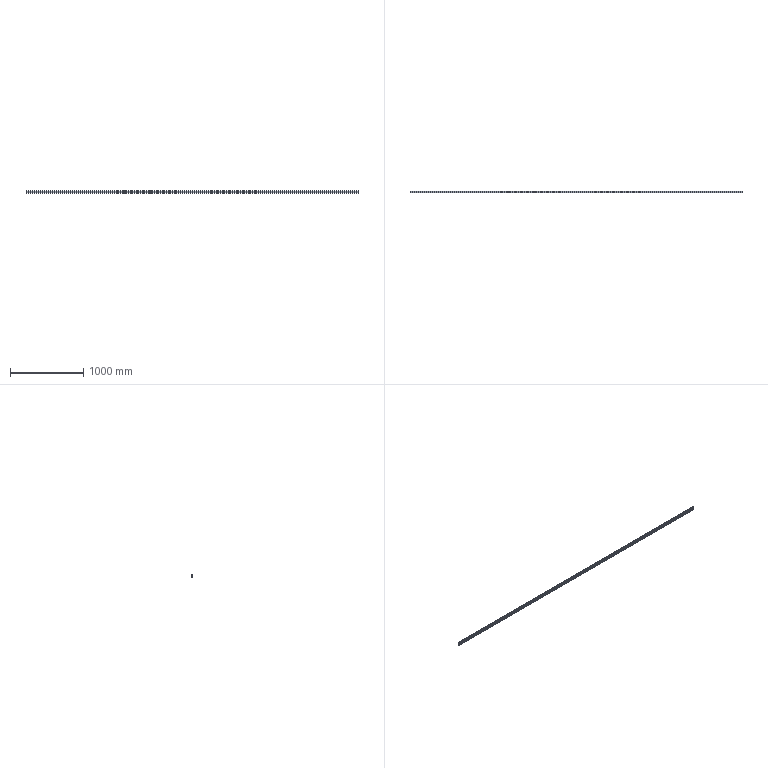Part | SolidWorks | features HoleWzd 1, WeldMemberFeat 1, WeldmentFeature 1 | 1 solid | 104 faces | box 4546 x 20 x 40 mm | volume 1364953 mm3 | plane 96 | cylinder 8 | commonest cylinder face diameters 3 x4 5 x4